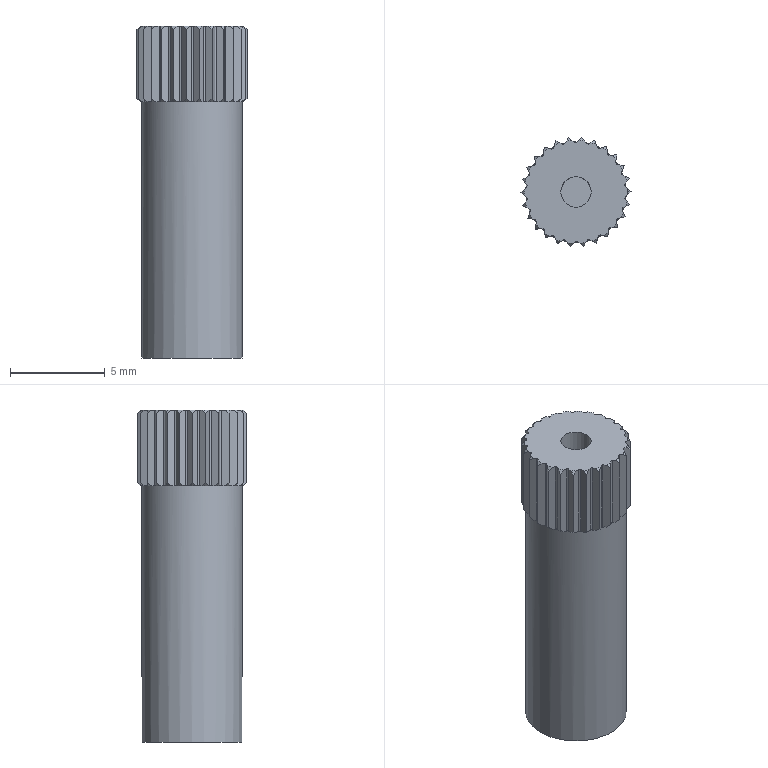Part | STEP file | Zapas-OpenRC Truggy HSPr v2. v55-4 | 1 solid | 189 faces | box 5.799 x 5.767 x 17.5 mm | volume 382.741 mm3 | plane 107 | cone 54 | cylinder 28 | commonest cylinder face diameters 5.2 x26 1.6 x1 5.3 x1